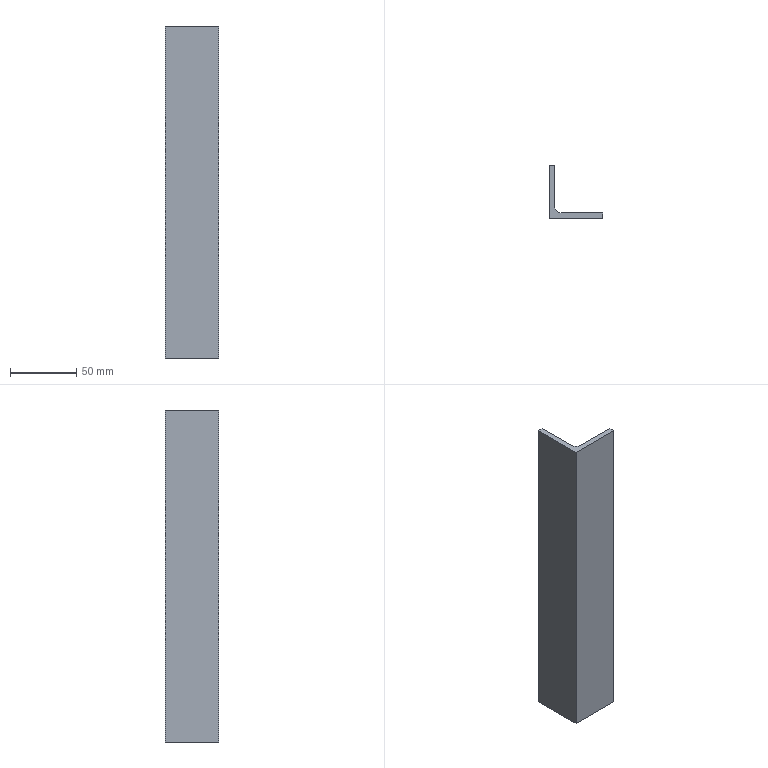Part | SolidWorks | features Extrusion 1 | 1 solid | 11 faces | box 40 x 40 x 250 mm | volume 77341 mm3 | plane 8 | cylinder 3 | commonest cylinder face diameters 0.02 x2 10 x1
STEP:
#1=CARTESIAN_POINT('',(0.,0.,0.));
#2=VERTEX_POINT('',#1);
#3=CARTESIAN_POINT('',(40.,0.,0.));
#4=VERTEX_POINT('',#3);
#5=CARTESIAN_POINT('',(40.,0.,0.));
#6=DIRECTION('',(1.,0.,0.));
#7=VECTOR('',#6,1000.);
#8=LINE('',#5,#7);
#9=EDGE_CURVE('',#2,#4,#8,.T.);
#10=ORIENTED_EDGE('',*,*,#9,.T.);
#11=CARTESIAN_POINT('',(40.,0.,250.));
#12=VERTEX_POINT('',#11);
#13=CARTESIAN_POINT('',(40.,0.,250.));
#14=DIRECTION('',(0.,0.,-1.));
#15=VECTOR('',#14,1000.);
#16=LINE('',#13,#15);
#17=EDGE_CURVE('',#12,#4,#16,.T.);
#18=ORIENTED_EDGE('',*,*,#17,.F.);
#19=CARTESIAN_POINT('',(0.,0.,250.));
#20=VERTEX_POINT('',#19);
#21=CARTESIAN_POINT('',(40.,0.,250.));
#22=DIRECTION('',(1.,0.,0.));
#23=VECTOR('',#22,1000.);
#24=LINE('',#21,#23);
#25=EDGE_CURVE('',#20,#12,#24,.T.);
#26=ORIENTED_EDGE('',*,*,#25,.F.);
#27=CARTESIAN_POINT('',(0.,0.,250.));
#28=DIRECTION('',(0.,0.,-1.));
#29=VECTOR('',#28,1000.);
#30=LINE('',#27,#29);
#31=EDGE_CURVE('',#20,#2,#30,.T.);
#32=ORIENTED_EDGE('',*,*,#31,.T.);
#33=EDGE_LOOP('',(#10,#18,#26,#32));
#34=FACE_OUTER_BOUND('',#33,.T.);
#35=CARTESIAN_POINT('',(40.,0.,250.));
#36=DIRECTION('',(0.,1.,0.));
#37=DIRECTION('',(-1.,0.,0.));
#38=AXIS2_PLACEMENT_3D('',#35,#36,#37);
#39=PLANE('',#38);
#40=ADVANCED_FACE('',(#34),#39,.F.);
#41=CARTESIAN_POINT('',(40.,3.99,0.));
#42=VERTEX_POINT('',#41);
#43=CARTESIAN_POINT('',(40.,3.99,0.));
#44=DIRECTION('',(0.,1.,0.));
#45=VECTOR('',#44,1000.);
#46=LINE('',#43,#45);
#47=EDGE_CURVE('',#4,#42,#46,.T.);
#48=ORIENTED_EDGE('',*,*,#47,.T.);
#49=CARTESIAN_POINT('',(40.,3.99,250.));
#50=VERTEX_POINT('',#49);
#51=CARTESIAN_POINT('',(40.,3.99,250.));
#52=DIRECTION('',(0.,0.,-1.));
#53=VECTOR('',#52,1000.);
#54=LINE('',#51,#53);
#55=EDGE_CURVE('',#50,#42,#54,.T.);
#56=ORIENTED_EDGE('',*,*,#55,.F.);
#57=CARTESIAN_POINT('',(40.,3.99,250.));
#58=DIRECTION('',(0.,1.,0.));
#59=VECTOR('',#58,1000.);
#60=LINE('',#57,#59);
#61=EDGE_CURVE('',#12,#50,#60,.T.);
#62=ORIENTED_EDGE('',*,*,#61,.F.);
#63=ORIENTED_EDGE('',*,*,#17,.T.);
#64=EDGE_LOOP('',(#48,#56,#62,#63));
#65=FACE_OUTER_BOUND('',#64,.T.);
#66=CARTESIAN_POINT('',(40.,3.99,250.));
#67=DIRECTION('',(-1.,0.,0.));
#68=DIRECTION('',(0.,-1.,0.));
#69=AXIS2_PLACEMENT_3D('',#66,#67,#68);
#70=PLANE('',#69);
#71=ADVANCED_FACE('',(#65),#70,.F.);
#72=CARTESIAN_POINT('',(39.99,4.,0.));
#73=VERTEX_POINT('',#72);
#74=CARTESIAN_POINT('',(39.99,3.99,0.));
#75=DIRECTION('',(0.,0.,1.));
#76=DIRECTION('',(1.,0.,0.));
#77=AXIS2_PLACEMENT_3D('',#74,#75,#76);
#78=CIRCLE('',#77,0.01);
#79=EDGE_CURVE('',#42,#73,#78,.T.);
#80=ORIENTED_EDGE('',*,*,#79,.T.);
#81=CARTESIAN_POINT('',(39.99,4.,250.));
#82=VERTEX_POINT('',#81);
#83=CARTESIAN_POINT('',(39.99,4.,250.));
#84=DIRECTION('',(0.,0.,-1.));
#85=VECTOR('',#84,1000.);
#86=LINE('',#83,#85);
#87=EDGE_CURVE('',#82,#73,#86,.T.);
#88=ORIENTED_EDGE('',*,*,#87,.F.);
#89=CARTESIAN_POINT('',(39.99,3.99,250.));
#90=DIRECTION('',(0.,0.,1.));
#91=DIRECTION('',(1.,0.,0.));
#92=AXIS2_PLACEMENT_3D('',#89,#90,#91);
#93=CIRCLE('',#92,0.01);
#94=EDGE_CURVE('',#50,#82,#93,.T.);
#95=ORIENTED_EDGE('',*,*,#94,.F.);
#96=ORIENTED_EDGE('',*,*,#55,.T.);
#97=EDGE_LOOP('',(#80,#88,#95,#96));
#98=FACE_OUTER_BOUND('',#97,.T.);
#99=CARTESIAN_POINT('',(39.99,3.99,250.));
#100=DIRECTION('',(0.,0.,-1.));
#101=DIRECTION('',(-1.,0.,0.));
#102=AXIS2_PLACEMENT_3D('',#99,#100,#101);
#103=CYLINDRICAL_SURFACE('',#102,0.01);
#104=ADVANCED_FACE('',(#98),#103,.T.);
#105=CARTESIAN_POINT('',(9.,4.,0.));
#106=VERTEX_POINT('',#105);
#107=CARTESIAN_POINT('',(9.,4.,0.));
#108=DIRECTION('',(-1.,0.,0.));
#109=VECTOR('',#108,1000.);
#110=LINE('',#107,#109);
#111=EDGE_CURVE('',#73,#106,#110,.T.);
#112=ORIENTED_EDGE('',*,*,#111,.T.);
#113=CARTESIAN_POINT('',(9.,4.,250.));
#114=VERTEX_POINT('',#113);
#115=CARTESIAN_POINT('',(9.,4.,250.));
#116=DIRECTION('',(0.,0.,-1.));
#117=VECTOR('',#116,1000.);
#118=LINE('',#115,#117);
#119=EDGE_CURVE('',#114,#106,#118,.T.);
#120=ORIENTED_EDGE('',*,*,#119,.F.);
#121=CARTESIAN_POINT('',(9.,4.,250.));
#122=DIRECTION('',(-1.,0.,0.));
#123=VECTOR('',#122,1000.);
#124=LINE('',#121,#123);
#125=EDGE_CURVE('',#82,#114,#124,.T.);
#126=ORIENTED_EDGE('',*,*,#125,.F.);
#127=ORIENTED_EDGE('',*,*,#87,.T.);
#128=EDGE_LOOP('',(#112,#120,#126,#127));
#129=FACE_OUTER_BOUND('',#128,.T.);
#130=CARTESIAN_POINT('',(9.,4.,250.));
#131=DIRECTION('',(0.,-1.,0.));
#132=DIRECTION('',(0.,0.,-1.));
#133=AXIS2_PLACEMENT_3D('',#130,#131,#132);
#134=PLANE('',#133);
#135=ADVANCED_FACE('',(#129),#134,.F.);
#136=CARTESIAN_POINT('',(4.,9.,0.));
#137=VERTEX_POINT('',#136);
#138=CARTESIAN_POINT('',(9.,9.,0.));
#139=DIRECTION('',(0.,0.,-1.));
#140=DIRECTION('',(-1.,0.,0.));
#141=AXIS2_PLACEMENT_3D('',#138,#139,#140);
#142=CIRCLE('',#141,5.);
#143=EDGE_CURVE('',#106,#137,#142,.T.);
#144=ORIENTED_EDGE('',*,*,#143,.T.);
#145=CARTESIAN_POINT('',(4.,9.,250.));
#146=VERTEX_POINT('',#145);
#147=CARTESIAN_POINT('',(4.,9.,250.));
#148=DIRECTION('',(0.,0.,-1.));
#149=VECTOR('',#148,1000.);
#150=LINE('',#147,#149);
#151=EDGE_CURVE('',#146,#137,#150,.T.);
#152=ORIENTED_EDGE('',*,*,#151,.F.);
#153=CARTESIAN_POINT('',(9.,9.,250.));
#154=DIRECTION('',(0.,0.,-1.));
#155=DIRECTION('',(-1.,0.,0.));
#156=AXIS2_PLACEMENT_3D('',#153,#154,#155);
#157=CIRCLE('',#156,5.);
#158=EDGE_CURVE('',#114,#146,#157,.T.);
#159=ORIENTED_EDGE('',*,*,#158,.F.);
#160=ORIENTED_EDGE('',*,*,#119,.T.);
#161=EDGE_LOOP('',(#144,#152,#159,#160));
#162=FACE_OUTER_BOUND('',#161,.T.);
#163=CARTESIAN_POINT('',(9.,9.,250.));
#164=DIRECTION('',(0.,0.,-1.));
#165=DIRECTION('',(-1.,0.,0.));
#166=AXIS2_PLACEMENT_3D('',#163,#164,#165);
#167=CYLINDRICAL_SURFACE('',#166,5.);
#168=ADVANCED_FACE('',(#162),#167,.F.);
#169=CARTESIAN_POINT('',(4.,39.99,0.));
#170=VERTEX_POINT('',#169);
#171=CARTESIAN_POINT('',(4.,39.99,0.));
#172=DIRECTION('',(0.,1.,0.));
#173=VECTOR('',#172,1000.);
#174=LINE('',#171,#173);
#175=EDGE_CURVE('',#137,#170,#174,.T.);
#176=ORIENTED_EDGE('',*,*,#175,.T.);
#177=CARTESIAN_POINT('',(4.,39.99,250.));
#178=VERTEX_POINT('',#177);
#179=CARTESIAN_POINT('',(4.,39.99,250.));
#180=DIRECTION('',(0.,0.,-1.));
#181=VECTOR('',#180,1000.);
#182=LINE('',#179,#181);
#183=EDGE_CURVE('',#178,#170,#182,.T.);
#184=ORIENTED_EDGE('',*,*,#183,.F.);
#185=CARTESIAN_POINT('',(4.,39.99,250.));
#186=DIRECTION('',(0.,1.,0.));
#187=VECTOR('',#186,1000.);
#188=LINE('',#185,#187);
#189=EDGE_CURVE('',#146,#178,#188,.T.);
#190=ORIENTED_EDGE('',*,*,#189,.F.);
#191=ORIENTED_EDGE('',*,*,#151,.T.);
#192=EDGE_LOOP('',(#176,#184,#190,#191));
#193=FACE_OUTER_BOUND('',#192,.T.);
#194=CARTESIAN_POINT('',(4.,39.99,250.));
#195=DIRECTION('',(-1.,0.,0.));
#196=DIRECTION('',(0.,-1.,0.));
#197=AXIS2_PLACEMENT_3D('',#194,#195,#196);
#198=PLANE('',#197);
#199=ADVANCED_FACE('',(#193),#198,.F.);
#200=CARTESIAN_POINT('',(3.99,40.,0.));
#201=VERTEX_POINT('',#200);
#202=CARTESIAN_POINT('',(3.99,39.99,0.));
#203=DIRECTION('',(0.,0.,1.));
#204=DIRECTION('',(1.,0.,0.));
#205=AXIS2_PLACEMENT_3D('',#202,#203,#204);
#206=CIRCLE('',#205,0.01);
#207=EDGE_CURVE('',#170,#201,#206,.T.);
#208=ORIENTED_EDGE('',*,*,#207,.T.);
#209=CARTESIAN_POINT('',(3.99,40.,250.));
#210=VERTEX_POINT('',#209);
#211=CARTESIAN_POINT('',(3.99,40.,250.));
#212=DIRECTION('',(0.,0.,-1.));
#213=VECTOR('',#212,1000.);
#214=LINE('',#211,#213);
#215=EDGE_CURVE('',#210,#201,#214,.T.);
#216=ORIENTED_EDGE('',*,*,#215,.F.);
#217=CARTESIAN_POINT('',(3.99,39.99,250.));
#218=DIRECTION('',(0.,0.,1.));
#219=DIRECTION('',(1.,0.,0.));
#220=AXIS2_PLACEMENT_3D('',#217,#218,#219);
#221=CIRCLE('',#220,0.01);
#222=EDGE_CURVE('',#178,#210,#221,.T.);
#223=ORIENTED_EDGE('',*,*,#222,.F.);
#224=ORIENTED_EDGE('',*,*,#183,.T.);
#225=EDGE_LOOP('',(#208,#216,#223,#224));
#226=FACE_OUTER_BOUND('',#225,.T.);
#227=CARTESIAN_POINT('',(3.99,39.99,250.));
#228=DIRECTION('',(0.,0.,-1.));
#229=DIRECTION('',(-1.,0.,0.));
#230=AXIS2_PLACEMENT_3D('',#227,#228,#229);
#231=CYLINDRICAL_SURFACE('',#230,0.01);
#232=ADVANCED_FACE('',(#226),#231,.T.);
#233=CARTESIAN_POINT('',(0.,40.,0.));
#234=VERTEX_POINT('',#233);
#235=CARTESIAN_POINT('',(0.,40.,0.));
#236=DIRECTION('',(-1.,0.,0.));
#237=VECTOR('',#236,1000.);
#238=LINE('',#235,#237);
#239=EDGE_CURVE('',#201,#234,#238,.T.);
#240=ORIENTED_EDGE('',*,*,#239,.T.);
#241=CARTESIAN_POINT('',(0.,40.,250.));
#242=VERTEX_POINT('',#241);
#243=CARTESIAN_POINT('',(0.,40.,250.));
#244=DIRECTION('',(0.,0.,-1.));
#245=VECTOR('',#244,1000.);
#246=LINE('',#243,#245);
#247=EDGE_CURVE('',#242,#234,#246,.T.);
#248=ORIENTED_EDGE('',*,*,#247,.F.);
#249=CARTESIAN_POINT('',(0.,40.,250.));
#250=DIRECTION('',(-1.,0.,0.));
#251=VECTOR('',#250,1000.);
#252=LINE('',#249,#251);
#253=EDGE_CURVE('',#210,#242,#252,.T.);
#254=ORIENTED_EDGE('',*,*,#253,.F.);
#255=ORIENTED_EDGE('',*,*,#215,.T.);
#256=EDGE_LOOP('',(#240,#248,#254,#255));
#257=FACE_OUTER_BOUND('',#256,.T.);
#258=CARTESIAN_POINT('',(0.,40.,250.));
#259=DIRECTION('',(0.,-1.,0.));
#260=DIRECTION('',(0.,0.,-1.));
#261=AXIS2_PLACEMENT_3D('',#258,#259,#260);
#262=PLANE('',#261);
#263=ADVANCED_FACE('',(#257),#262,.F.);
#264=CARTESIAN_POINT('',(0.,0.,0.));
#265=DIRECTION('',(0.,-1.,0.));
#266=VECTOR('',#265,1000.);
#267=LINE('',#264,#266);
#268=EDGE_CURVE('',#234,#2,#267,.T.);
#269=ORIENTED_EDGE('',*,*,#268,.T.);
#270=ORIENTED_EDGE('',*,*,#31,.F.);
#271=CARTESIAN_POINT('',(0.,0.,250.));
#272=DIRECTION('',(0.,-1.,0.));
#273=VECTOR('',#272,1000.);
#274=LINE('',#271,#273);
#275=EDGE_CURVE('',#242,#20,#274,.T.);
#276=ORIENTED_EDGE('',*,*,#275,.F.);
#277=ORIENTED_EDGE('',*,*,#247,.T.);
#278=EDGE_LOOP('',(#269,#270,#276,#277));
#279=FACE_OUTER_BOUND('',#278,.T.);
#280=CARTESIAN_POINT('',(0.,0.,250.));
#281=DIRECTION('',(1.,0.,0.));
#282=DIRECTION('',(0.,0.,-1.));
#283=AXIS2_PLACEMENT_3D('',#280,#281,#282);
#284=PLANE('',#283);
#285=ADVANCED_FACE('',(#279),#284,.F.);
#286=ORIENTED_EDGE('',*,*,#25,.T.);
#287=ORIENTED_EDGE('',*,*,#61,.T.);
#288=ORIENTED_EDGE('',*,*,#94,.T.);
#289=ORIENTED_EDGE('',*,*,#125,.T.);
#290=ORIENTED_EDGE('',*,*,#158,.T.);
#291=ORIENTED_EDGE('',*,*,#189,.T.);
#292=ORIENTED_EDGE('',*,*,#222,.T.);
#293=ORIENTED_EDGE('',*,*,#253,.T.);
#294=ORIENTED_EDGE('',*,*,#275,.T.);
#295=EDGE_LOOP('',(#286,#287,#288,#289,#290,#291,#292,#293,#294));
#296=FACE_OUTER_BOUND('',#295,.T.);
#297=CARTESIAN_POINT('',(3.99,39.99,250.));
#298=DIRECTION('',(0.,0.,1.));
#299=DIRECTION('',(1.,0.,0.));
#300=AXIS2_PLACEMENT_3D('',#297,#298,#299);
#301=PLANE('',#300);
#302=ADVANCED_FACE('',(#296),#301,.T.);
#303=ORIENTED_EDGE('',*,*,#9,.F.);
#304=ORIENTED_EDGE('',*,*,#268,.F.);
#305=ORIENTED_EDGE('',*,*,#239,.F.);
#306=ORIENTED_EDGE('',*,*,#207,.F.);
#307=ORIENTED_EDGE('',*,*,#175,.F.);
#308=ORIENTED_EDGE('',*,*,#143,.F.);
#309=ORIENTED_EDGE('',*,*,#111,.F.);
#310=ORIENTED_EDGE('',*,*,#79,.F.);
#311=ORIENTED_EDGE('',*,*,#47,.F.);
#312=EDGE_LOOP('',(#303,#304,#305,#306,#307,#308,#309,#310,#311));
#313=FACE_OUTER_BOUND('',#312,.T.);
#314=CARTESIAN_POINT('',(3.99,39.99,0.));
#315=DIRECTION('',(0.,0.,1.));
#316=DIRECTION('',(1.,0.,0.));
#317=AXIS2_PLACEMENT_3D('',#314,#315,#316);
#318=PLANE('',#317);
#319=ADVANCED_FACE('',(#313),#318,.F.);
#320=CLOSED_SHELL('',(#40,#71,#104,#135,#168,#199,#232,#263,#285,#302,#319));
#321=MANIFOLD_SOLID_BREP('',#320);
#322=CARTESIAN_POINT('',(0.,0.,0.));
#323=DIRECTION('',(0.,0.,1.));
#324=DIRECTION('',(1.,0.,0.));
#325=AXIS2_PLACEMENT_3D('',#322,#323,#324);
#326=(LENGTH_UNIT()NAMED_UNIT(*)SI_UNIT(.MILLI.,.METRE.));
#327=UNCERTAINTY_MEASURE_WITH_UNIT(LENGTH_MEASURE(0.00001),#326,'','');
#328=(NAMED_UNIT(*)PLANE_ANGLE_UNIT()SI_UNIT($,.RADIAN.));
#329=(NAMED_UNIT(*)SI_UNIT($,.STERADIAN.)SOLID_ANGLE_UNIT());
#330=(GEOMETRIC_REPRESENTATION_CONTEXT(3)GLOBAL_UNCERTAINTY_ASSIGNED_CONTEXT((#327))GLOBAL_UNIT_ASSIGNED_CONTEXT((#326,#328,#329))REPRESENTATION_CONTEXT('',''));
#331=ADVANCED_BREP_SHAPE_REPRESENTATION('',(#321,#325),#330);